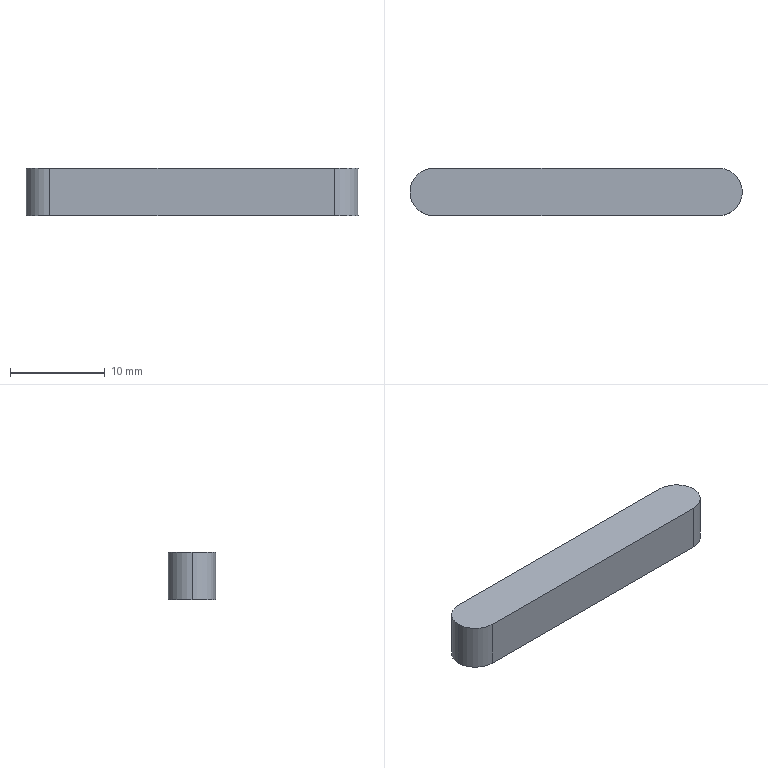Part | SolidWorks | features Extrusion 1 | 1 solid | 7 faces | box 35 x 5 x 5 mm | volume 848.175 mm3 | plane 4 | cylinder 3 | commonest cylinder face diameters 5 x3
STEP:
#1=CARTESIAN_POINT('',(-17.5,0.,5.));
#2=VERTEX_POINT('',#1);
#3=CARTESIAN_POINT('',(-15.,-2.5,5.));
#4=VERTEX_POINT('',#3);
#5=CARTESIAN_POINT('',(-15.,0.,5.));
#6=DIRECTION('',(0.,0.,1.));
#7=DIRECTION('',(1.,0.,0.));
#8=AXIS2_PLACEMENT_3D('',#5,#6,#7);
#9=CIRCLE('',#8,2.5);
#10=EDGE_CURVE('',#2,#4,#9,.T.);
#11=ORIENTED_EDGE('',*,*,#10,.F.);
#12=CARTESIAN_POINT('',(-17.5,0.,0.));
#13=VERTEX_POINT('',#12);
#14=CARTESIAN_POINT('',(-17.5,0.,5.));
#15=DIRECTION('',(0.,0.,-1.));
#16=VECTOR('',#15,1000.);
#17=LINE('',#14,#16);
#18=EDGE_CURVE('',#2,#13,#17,.T.);
#19=ORIENTED_EDGE('',*,*,#18,.T.);
#20=CARTESIAN_POINT('',(-15.,-2.5,0.));
#21=VERTEX_POINT('',#20);
#22=CARTESIAN_POINT('',(-15.,0.,0.));
#23=DIRECTION('',(0.,0.,1.));
#24=DIRECTION('',(1.,0.,0.));
#25=AXIS2_PLACEMENT_3D('',#22,#23,#24);
#26=CIRCLE('',#25,2.5);
#27=EDGE_CURVE('',#13,#21,#26,.T.);
#28=ORIENTED_EDGE('',*,*,#27,.T.);
#29=CARTESIAN_POINT('',(-15.,-2.5,5.));
#30=DIRECTION('',(0.,0.,-1.));
#31=VECTOR('',#30,1000.);
#32=LINE('',#29,#31);
#33=EDGE_CURVE('',#4,#21,#32,.T.);
#34=ORIENTED_EDGE('',*,*,#33,.F.);
#35=EDGE_LOOP('',(#11,#19,#28,#34));
#36=FACE_OUTER_BOUND('',#35,.T.);
#37=CARTESIAN_POINT('',(-15.,0.,5.));
#38=DIRECTION('',(0.,0.,-1.));
#39=DIRECTION('',(-1.,0.,0.));
#40=AXIS2_PLACEMENT_3D('',#37,#38,#39);
#41=CYLINDRICAL_SURFACE('',#40,2.5);
#42=ADVANCED_FACE('',(#36),#41,.T.);
#43=ORIENTED_EDGE('',*,*,#18,.F.);
#44=CARTESIAN_POINT('',(-15.,2.5,5.));
#45=VERTEX_POINT('',#44);
#46=CARTESIAN_POINT('',(-15.,0.,5.));
#47=DIRECTION('',(0.,0.,1.));
#48=DIRECTION('',(1.,0.,0.));
#49=AXIS2_PLACEMENT_3D('',#46,#47,#48);
#50=CIRCLE('',#49,2.5);
#51=EDGE_CURVE('',#45,#2,#50,.T.);
#52=ORIENTED_EDGE('',*,*,#51,.F.);
#53=CARTESIAN_POINT('',(-15.,2.5,0.));
#54=VERTEX_POINT('',#53);
#55=CARTESIAN_POINT('',(-15.,2.5,5.));
#56=DIRECTION('',(0.,0.,-1.));
#57=VECTOR('',#56,1000.);
#58=LINE('',#55,#57);
#59=EDGE_CURVE('',#45,#54,#58,.T.);
#60=ORIENTED_EDGE('',*,*,#59,.T.);
#61=CARTESIAN_POINT('',(-15.,0.,0.));
#62=DIRECTION('',(0.,0.,1.));
#63=DIRECTION('',(1.,0.,0.));
#64=AXIS2_PLACEMENT_3D('',#61,#62,#63);
#65=CIRCLE('',#64,2.5);
#66=EDGE_CURVE('',#54,#13,#65,.T.);
#67=ORIENTED_EDGE('',*,*,#66,.T.);
#68=EDGE_LOOP('',(#43,#52,#60,#67));
#69=FACE_OUTER_BOUND('',#68,.T.);
#70=CARTESIAN_POINT('',(-15.,0.,5.));
#71=DIRECTION('',(0.,0.,-1.));
#72=DIRECTION('',(-1.,0.,0.));
#73=AXIS2_PLACEMENT_3D('',#70,#71,#72);
#74=CYLINDRICAL_SURFACE('',#73,2.5);
#75=ADVANCED_FACE('',(#69),#74,.T.);
#76=CARTESIAN_POINT('',(15.,-2.5,0.));
#77=VERTEX_POINT('',#76);
#78=CARTESIAN_POINT('',(-15.,-2.5,0.));
#79=DIRECTION('',(1.,0.,0.));
#80=VECTOR('',#79,1000.);
#81=LINE('',#78,#80);
#82=EDGE_CURVE('',#21,#77,#81,.T.);
#83=ORIENTED_EDGE('',*,*,#82,.T.);
#84=CARTESIAN_POINT('',(15.,-2.5,5.));
#85=VERTEX_POINT('',#84);
#86=CARTESIAN_POINT('',(15.,-2.5,5.));
#87=DIRECTION('',(0.,0.,-1.));
#88=VECTOR('',#87,1000.);
#89=LINE('',#86,#88);
#90=EDGE_CURVE('',#85,#77,#89,.T.);
#91=ORIENTED_EDGE('',*,*,#90,.F.);
#92=CARTESIAN_POINT('',(-15.,-2.5,5.));
#93=DIRECTION('',(1.,0.,0.));
#94=VECTOR('',#93,1000.);
#95=LINE('',#92,#94);
#96=EDGE_CURVE('',#4,#85,#95,.T.);
#97=ORIENTED_EDGE('',*,*,#96,.F.);
#98=ORIENTED_EDGE('',*,*,#33,.T.);
#99=EDGE_LOOP('',(#83,#91,#97,#98));
#100=FACE_OUTER_BOUND('',#99,.T.);
#101=CARTESIAN_POINT('',(-15.,-2.5,5.));
#102=DIRECTION('',(0.,1.,0.));
#103=DIRECTION('',(-1.,0.,0.));
#104=AXIS2_PLACEMENT_3D('',#101,#102,#103);
#105=PLANE('',#104);
#106=ADVANCED_FACE('',(#100),#105,.F.);
#107=CARTESIAN_POINT('',(15.,2.5,0.));
#108=VERTEX_POINT('',#107);
#109=CARTESIAN_POINT('',(15.,0.,0.));
#110=DIRECTION('',(0.,0.,1.));
#111=DIRECTION('',(1.,0.,0.));
#112=AXIS2_PLACEMENT_3D('',#109,#110,#111);
#113=CIRCLE('',#112,2.5);
#114=EDGE_CURVE('',#77,#108,#113,.T.);
#115=ORIENTED_EDGE('',*,*,#114,.T.);
#116=CARTESIAN_POINT('',(15.,2.5,5.));
#117=VERTEX_POINT('',#116);
#118=CARTESIAN_POINT('',(15.,2.5,5.));
#119=DIRECTION('',(0.,0.,-1.));
#120=VECTOR('',#119,1000.);
#121=LINE('',#118,#120);
#122=EDGE_CURVE('',#117,#108,#121,.T.);
#123=ORIENTED_EDGE('',*,*,#122,.F.);
#124=CARTESIAN_POINT('',(15.,0.,5.));
#125=DIRECTION('',(0.,0.,1.));
#126=DIRECTION('',(1.,0.,0.));
#127=AXIS2_PLACEMENT_3D('',#124,#125,#126);
#128=CIRCLE('',#127,2.5);
#129=EDGE_CURVE('',#85,#117,#128,.T.);
#130=ORIENTED_EDGE('',*,*,#129,.F.);
#131=ORIENTED_EDGE('',*,*,#90,.T.);
#132=EDGE_LOOP('',(#115,#123,#130,#131));
#133=FACE_OUTER_BOUND('',#132,.T.);
#134=CARTESIAN_POINT('',(15.,0.,5.));
#135=DIRECTION('',(0.,0.,-1.));
#136=DIRECTION('',(-1.,0.,0.));
#137=AXIS2_PLACEMENT_3D('',#134,#135,#136);
#138=CYLINDRICAL_SURFACE('',#137,2.5);
#139=ADVANCED_FACE('',(#133),#138,.T.);
#140=CARTESIAN_POINT('',(-15.,2.5,0.));
#141=DIRECTION('',(-1.,0.,0.));
#142=VECTOR('',#141,1000.);
#143=LINE('',#140,#142);
#144=EDGE_CURVE('',#108,#54,#143,.T.);
#145=ORIENTED_EDGE('',*,*,#144,.T.);
#146=ORIENTED_EDGE('',*,*,#59,.F.);
#147=CARTESIAN_POINT('',(-15.,2.5,5.));
#148=DIRECTION('',(-1.,0.,0.));
#149=VECTOR('',#148,1000.);
#150=LINE('',#147,#149);
#151=EDGE_CURVE('',#117,#45,#150,.T.);
#152=ORIENTED_EDGE('',*,*,#151,.F.);
#153=ORIENTED_EDGE('',*,*,#122,.T.);
#154=EDGE_LOOP('',(#145,#146,#152,#153));
#155=FACE_OUTER_BOUND('',#154,.T.);
#156=CARTESIAN_POINT('',(-15.,2.5,5.));
#157=DIRECTION('',(0.,-1.,0.));
#158=DIRECTION('',(1.,0.,0.));
#159=AXIS2_PLACEMENT_3D('',#156,#157,#158);
#160=PLANE('',#159);
#161=ADVANCED_FACE('',(#155),#160,.F.);
#162=ORIENTED_EDGE('',*,*,#51,.T.);
#163=ORIENTED_EDGE('',*,*,#10,.T.);
#164=ORIENTED_EDGE('',*,*,#96,.T.);
#165=ORIENTED_EDGE('',*,*,#129,.T.);
#166=ORIENTED_EDGE('',*,*,#151,.T.);
#167=EDGE_LOOP('',(#162,#163,#164,#165,#166));
#168=FACE_OUTER_BOUND('',#167,.T.);
#169=CARTESIAN_POINT('',(-15.,0.,5.));
#170=DIRECTION('',(0.,0.,1.));
#171=DIRECTION('',(1.,0.,0.));
#172=AXIS2_PLACEMENT_3D('',#169,#170,#171);
#173=PLANE('',#172);
#174=ADVANCED_FACE('',(#168),#173,.T.);
#175=ORIENTED_EDGE('',*,*,#66,.F.);
#176=ORIENTED_EDGE('',*,*,#144,.F.);
#177=ORIENTED_EDGE('',*,*,#114,.F.);
#178=ORIENTED_EDGE('',*,*,#82,.F.);
#179=ORIENTED_EDGE('',*,*,#27,.F.);
#180=EDGE_LOOP('',(#175,#176,#177,#178,#179));
#181=FACE_OUTER_BOUND('',#180,.T.);
#182=CARTESIAN_POINT('',(-15.,0.,0.));
#183=DIRECTION('',(0.,0.,1.));
#184=DIRECTION('',(1.,0.,0.));
#185=AXIS2_PLACEMENT_3D('',#182,#183,#184);
#186=PLANE('',#185);
#187=ADVANCED_FACE('',(#181),#186,.F.);
#188=CLOSED_SHELL('',(#42,#75,#106,#139,#161,#174,#187));
#189=MANIFOLD_SOLID_BREP('',#188);
#190=CARTESIAN_POINT('',(0.,0.,0.));
#191=DIRECTION('',(0.,0.,1.));
#192=DIRECTION('',(1.,0.,0.));
#193=AXIS2_PLACEMENT_3D('',#190,#191,#192);
#194=(LENGTH_UNIT()NAMED_UNIT(*)SI_UNIT(.MILLI.,.METRE.));
#195=UNCERTAINTY_MEASURE_WITH_UNIT(LENGTH_MEASURE(0.00001),#194,'','');
#196=(NAMED_UNIT(*)PLANE_ANGLE_UNIT()SI_UNIT($,.RADIAN.));
#197=(NAMED_UNIT(*)SI_UNIT($,.STERADIAN.)SOLID_ANGLE_UNIT());
#198=(GEOMETRIC_REPRESENTATION_CONTEXT(3)GLOBAL_UNCERTAINTY_ASSIGNED_CONTEXT((#195))GLOBAL_UNIT_ASSIGNED_CONTEXT((#194,#196,#197))REPRESENTATION_CONTEXT('',''));
#199=ADVANCED_BREP_SHAPE_REPRESENTATION('',(#189,#193),#198);